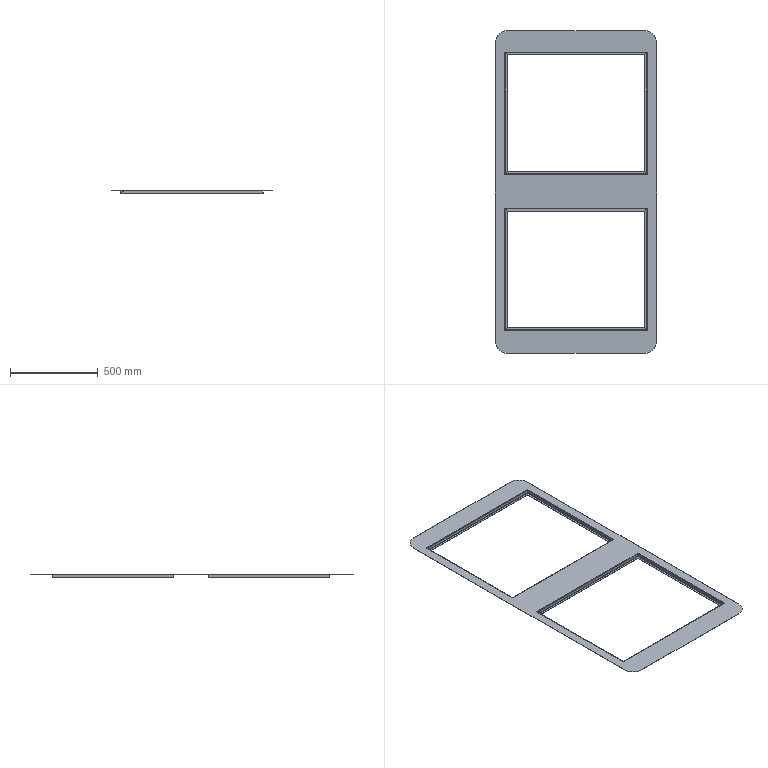Part | STEP file | Split housing part 0401001 | 1 solid | 154 faces | box 920 x 1840 x 21.5 mm | volume 1137707 mm3 | plane 78 | cylinder 44 | spline 32 | commonest cylinder face diameters 3 x16 6 x16 5 x8 140 x4